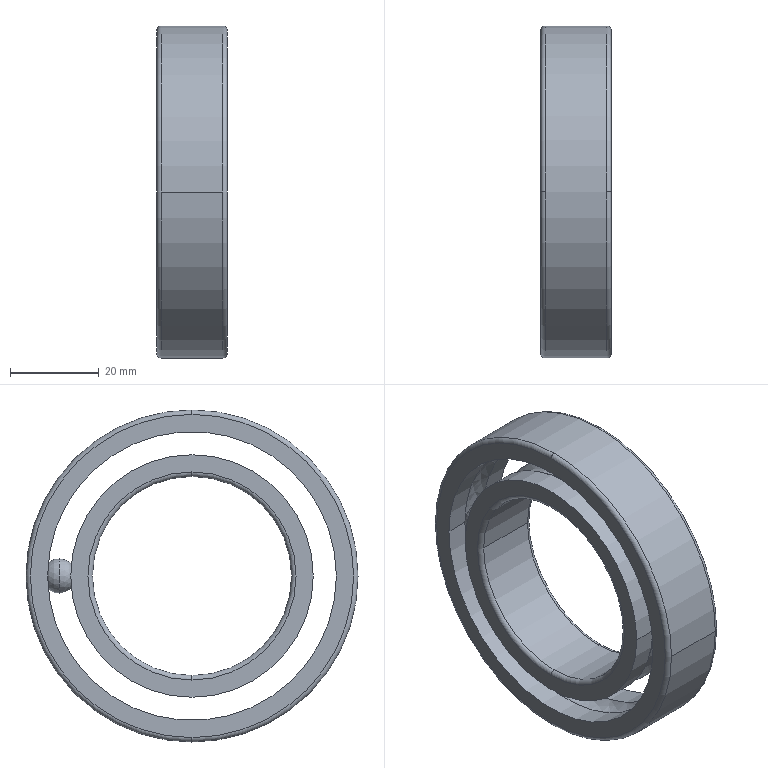Part | STEP file | PN_0027_default | 3 solids | 30 faces | box 16 x 75 x 75 mm | volume 27632 mm3 | cylinder 12 | torus 8 | plane 4 | spline 4 | sphere 2 | commonest cylinder face diameters 54.78 x4 65.22 x4 45 x2 75 x2